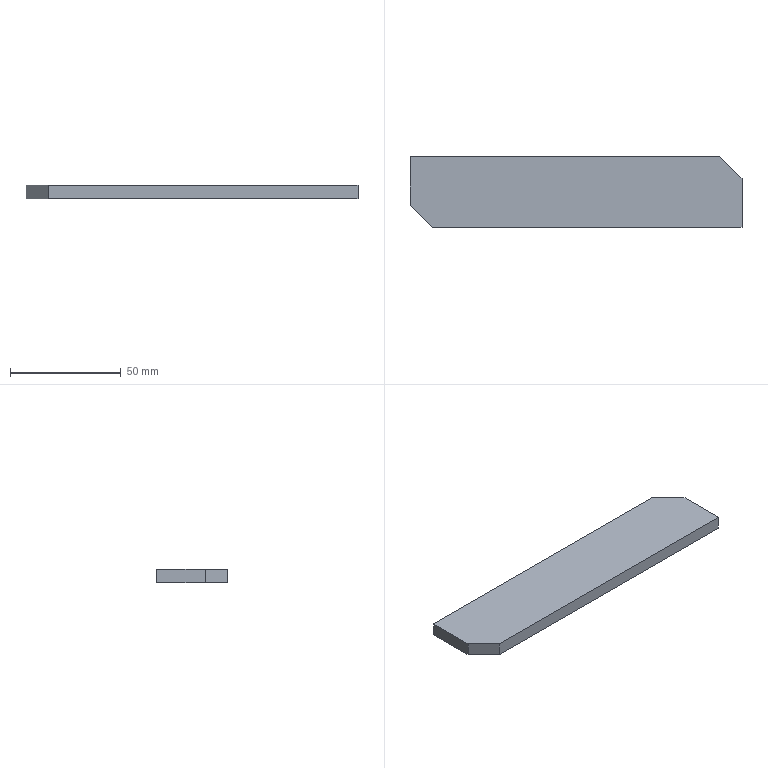Part | STEP file | [02]-7 | 1 solid | 8 faces | box 150 x 32 x 6 mm | volume 28200 mm3 | plane 8
STEP:
#1=CARTESIAN_POINT('',(0.,0.,0.));
#2=DIRECTION('',(0.,0.,1.));
#3=DIRECTION('',(1.,0.,0.));
#4=AXIS2_PLACEMENT_3D('',#1,#2,#3);
#5=CARTESIAN_POINT('',(0.,-22.,0.));
#6=VERTEX_POINT('',#5);
#7=CARTESIAN_POINT('',(0.,0.,0.));
#8=VERTEX_POINT('',#7);
#9=CARTESIAN_POINT('',(0.,-16.,0.));
#10=DIRECTION('',(0.,1.,0.));
#11=VECTOR('',#10,1.);
#12=LINE('',#9,#11);
#13=CARTESIAN_POINT('',(75.,-16.,0.));
#14=DIRECTION('',(0.,0.,-1.));
#15=DIRECTION('',(0.,-1.,0.));
#16=AXIS2_PLACEMENT_3D('',#13,#14,#15);
#17=PLANE('',#16);
#18=CARTESIAN_POINT('',(0.,75.));
#19=DIRECTION('',(-1.,0.));
#20=VECTOR('',#19,1.);
#21=LINE('',#18,#20);
#22=(GEOMETRIC_REPRESENTATION_CONTEXT(2)PARAMETRIC_REPRESENTATION_CONTEXT()REPRESENTATION_CONTEXT('',''));
#23=DEFINITIONAL_REPRESENTATION('',(#21),#22);
#24=PCURVE('',#17,#23);
#25=CARTESIAN_POINT('',(0.,-16.,6.));
#26=DIRECTION('',(-1.,0.,0.));
#27=DIRECTION('',(0.,0.,1.));
#28=AXIS2_PLACEMENT_3D('',#25,#26,#27);
#29=PLANE('',#28);
#30=CARTESIAN_POINT('',(-6.,0.));
#31=DIRECTION('',(0.,1.));
#32=VECTOR('',#31,1.);
#33=LINE('',#30,#32);
#34=(GEOMETRIC_REPRESENTATION_CONTEXT(2)PARAMETRIC_REPRESENTATION_CONTEXT()REPRESENTATION_CONTEXT('',''));
#35=DEFINITIONAL_REPRESENTATION('',(#33),#34);
#36=PCURVE('',#29,#35);
#37=SURFACE_CURVE('',#12,(#24,#36),.PCURVE_S1.);
#38=EDGE_CURVE('',#6,#8,#37,.T.);
#39=ORIENTED_EDGE('',*,*,#38,.T.);
#40=CARTESIAN_POINT('',(140.,0.,0.));
#41=VERTEX_POINT('',#40);
#42=CARTESIAN_POINT('',(75.,0.,0.));
#43=DIRECTION('',(1.,0.,0.));
#44=VECTOR('',#43,1.);
#45=LINE('',#42,#44);
#46=CARTESIAN_POINT('',(-16.,0.));
#47=DIRECTION('',(0.,-1.));
#48=VECTOR('',#47,1.);
#49=LINE('',#46,#48);
#50=(GEOMETRIC_REPRESENTATION_CONTEXT(2)PARAMETRIC_REPRESENTATION_CONTEXT()REPRESENTATION_CONTEXT('',''));
#51=DEFINITIONAL_REPRESENTATION('',(#49),#50);
#52=PCURVE('',#17,#51);
#53=CARTESIAN_POINT('',(75.,0.,6.));
#54=DIRECTION('',(0.,1.,0.));
#55=DIRECTION('',(0.,0.,-1.));
#56=AXIS2_PLACEMENT_3D('',#53,#54,#55);
#57=PLANE('',#56);
#58=CARTESIAN_POINT('',(6.,0.));
#59=DIRECTION('',(0.,-1.));
#60=VECTOR('',#59,1.);
#61=LINE('',#58,#60);
#62=(GEOMETRIC_REPRESENTATION_CONTEXT(2)PARAMETRIC_REPRESENTATION_CONTEXT()REPRESENTATION_CONTEXT('',''));
#63=DEFINITIONAL_REPRESENTATION('',(#61),#62);
#64=PCURVE('',#57,#63);
#65=SURFACE_CURVE('',#45,(#52,#64),.PCURVE_S1.);
#66=EDGE_CURVE('',#8,#41,#65,.T.);
#67=ORIENTED_EDGE('',*,*,#66,.T.);
#68=CARTESIAN_POINT('',(150.,-10.,0.));
#69=VERTEX_POINT('',#68);
#70=CARTESIAN_POINT('',(115.5,24.5,0.));
#71=DIRECTION('',(-0.7071,0.7071,0.));
#72=VECTOR('',#71,1.);
#73=LINE('',#70,#72);
#74=CARTESIAN_POINT('',(-40.5,-40.5));
#75=DIRECTION('',(-0.7071,0.7071));
#76=VECTOR('',#75,1.);
#77=LINE('',#74,#76);
#78=(GEOMETRIC_REPRESENTATION_CONTEXT(2)PARAMETRIC_REPRESENTATION_CONTEXT()REPRESENTATION_CONTEXT('',''));
#79=DEFINITIONAL_REPRESENTATION('',(#77),#78);
#80=PCURVE('',#17,#79);
#81=CARTESIAN_POINT('',(150.,-10.,6.));
#82=DIRECTION('',(-0.7071,-0.7071,0.));
#83=DIRECTION('',(0.,0.,-1.));
#84=AXIS2_PLACEMENT_3D('',#81,#82,#83);
#85=PLANE('',#84);
#86=CARTESIAN_POINT('',(6.,-48.79));
#87=DIRECTION('',(0.,-1.));
#88=VECTOR('',#87,1.);
#89=LINE('',#86,#88);
#90=(GEOMETRIC_REPRESENTATION_CONTEXT(2)PARAMETRIC_REPRESENTATION_CONTEXT()REPRESENTATION_CONTEXT('',''));
#91=DEFINITIONAL_REPRESENTATION('',(#89),#90);
#92=PCURVE('',#85,#91);
#93=SURFACE_CURVE('',#73,(#80,#92),.PCURVE_S1.);
#94=EDGE_CURVE('',#69,#41,#93,.T.);
#95=ORIENTED_EDGE('',*,*,#94,.F.);
#96=CARTESIAN_POINT('',(150.,-32.,0.));
#97=VERTEX_POINT('',#96);
#98=CARTESIAN_POINT('',(150.,-16.,0.));
#99=DIRECTION('',(0.,-1.,0.));
#100=VECTOR('',#99,1.);
#101=LINE('',#98,#100);
#102=CARTESIAN_POINT('',(0.,-75.));
#103=DIRECTION('',(1.,0.));
#104=VECTOR('',#103,1.);
#105=LINE('',#102,#104);
#106=(GEOMETRIC_REPRESENTATION_CONTEXT(2)PARAMETRIC_REPRESENTATION_CONTEXT()REPRESENTATION_CONTEXT('',''));
#107=DEFINITIONAL_REPRESENTATION('',(#105),#106);
#108=PCURVE('',#17,#107);
#109=CARTESIAN_POINT('',(150.,-16.,6.));
#110=DIRECTION('',(1.,0.,0.));
#111=DIRECTION('',(0.,0.,-1.));
#112=AXIS2_PLACEMENT_3D('',#109,#110,#111);
#113=PLANE('',#112);
#114=CARTESIAN_POINT('',(6.,0.));
#115=DIRECTION('',(0.,-1.));
#116=VECTOR('',#115,1.);
#117=LINE('',#114,#116);
#118=(GEOMETRIC_REPRESENTATION_CONTEXT(2)PARAMETRIC_REPRESENTATION_CONTEXT()REPRESENTATION_CONTEXT('',''));
#119=DEFINITIONAL_REPRESENTATION('',(#117),#118);
#120=PCURVE('',#113,#119);
#121=SURFACE_CURVE('',#101,(#108,#120),.PCURVE_S1.);
#122=EDGE_CURVE('',#69,#97,#121,.T.);
#123=ORIENTED_EDGE('',*,*,#122,.T.);
#124=CARTESIAN_POINT('',(10.,-32.,0.));
#125=VERTEX_POINT('',#124);
#126=CARTESIAN_POINT('',(75.,-32.,0.));
#127=DIRECTION('',(-1.,0.,0.));
#128=VECTOR('',#127,1.);
#129=LINE('',#126,#128);
#130=CARTESIAN_POINT('',(16.,0.));
#131=DIRECTION('',(0.,1.));
#132=VECTOR('',#131,1.);
#133=LINE('',#130,#132);
#134=(GEOMETRIC_REPRESENTATION_CONTEXT(2)PARAMETRIC_REPRESENTATION_CONTEXT()REPRESENTATION_CONTEXT('',''));
#135=DEFINITIONAL_REPRESENTATION('',(#133),#134);
#136=PCURVE('',#17,#135);
#137=CARTESIAN_POINT('',(75.,-32.,6.));
#138=DIRECTION('',(0.,-1.,0.));
#139=DIRECTION('',(0.,0.,1.));
#140=AXIS2_PLACEMENT_3D('',#137,#138,#139);
#141=PLANE('',#140);
#142=CARTESIAN_POINT('',(-6.,0.));
#143=DIRECTION('',(0.,1.));
#144=VECTOR('',#143,1.);
#145=LINE('',#142,#144);
#146=(GEOMETRIC_REPRESENTATION_CONTEXT(2)PARAMETRIC_REPRESENTATION_CONTEXT()REPRESENTATION_CONTEXT('',''));
#147=DEFINITIONAL_REPRESENTATION('',(#145),#146);
#148=PCURVE('',#141,#147);
#149=SURFACE_CURVE('',#129,(#136,#148),.PCURVE_S1.);
#150=EDGE_CURVE('',#97,#125,#149,.T.);
#151=ORIENTED_EDGE('',*,*,#150,.T.);
#152=CARTESIAN_POINT('',(34.5,-56.5,0.));
#153=DIRECTION('',(0.7071,-0.7071,0.));
#154=VECTOR('',#153,1.);
#155=LINE('',#152,#154);
#156=CARTESIAN_POINT('',(40.5,40.5));
#157=DIRECTION('',(0.7071,-0.7071));
#158=VECTOR('',#157,1.);
#159=LINE('',#156,#158);
#160=(GEOMETRIC_REPRESENTATION_CONTEXT(2)PARAMETRIC_REPRESENTATION_CONTEXT()REPRESENTATION_CONTEXT('',''));
#161=DEFINITIONAL_REPRESENTATION('',(#159),#160);
#162=PCURVE('',#17,#161);
#163=CARTESIAN_POINT('',(0.,-22.,6.));
#164=DIRECTION('',(0.7071,0.7071,0.));
#165=DIRECTION('',(0.,0.,-1.));
#166=AXIS2_PLACEMENT_3D('',#163,#164,#165);
#167=PLANE('',#166);
#168=CARTESIAN_POINT('',(6.,-48.79));
#169=DIRECTION('',(0.,-1.));
#170=VECTOR('',#169,1.);
#171=LINE('',#168,#170);
#172=(GEOMETRIC_REPRESENTATION_CONTEXT(2)PARAMETRIC_REPRESENTATION_CONTEXT()REPRESENTATION_CONTEXT('',''));
#173=DEFINITIONAL_REPRESENTATION('',(#171),#172);
#174=PCURVE('',#167,#173);
#175=SURFACE_CURVE('',#155,(#162,#174),.PCURVE_S1.);
#176=EDGE_CURVE('',#6,#125,#175,.T.);
#177=ORIENTED_EDGE('',*,*,#176,.F.);
#178=EDGE_LOOP('',(#39,#67,#95,#123,#151,#177));
#179=FACE_BOUND('',#178,.T.);
#180=ADVANCED_FACE('',(#179),#17,.T.);
#181=CARTESIAN_POINT('',(0.,0.,6.));
#182=VERTEX_POINT('',#181);
#183=CARTESIAN_POINT('',(0.,-22.,6.));
#184=VERTEX_POINT('',#183);
#185=CARTESIAN_POINT('',(0.,-16.,6.));
#186=DIRECTION('',(0.,-1.,0.));
#187=VECTOR('',#186,1.);
#188=LINE('',#185,#187);
#189=CARTESIAN_POINT('',(0.,0.));
#190=DIRECTION('',(0.,-1.));
#191=VECTOR('',#190,1.);
#192=LINE('',#189,#191);
#193=(GEOMETRIC_REPRESENTATION_CONTEXT(2)PARAMETRIC_REPRESENTATION_CONTEXT()REPRESENTATION_CONTEXT('',''));
#194=DEFINITIONAL_REPRESENTATION('',(#192),#193);
#195=PCURVE('',#29,#194);
#196=CARTESIAN_POINT('',(75.,-16.,6.));
#197=DIRECTION('',(0.,0.,1.));
#198=DIRECTION('',(0.,1.,0.));
#199=AXIS2_PLACEMENT_3D('',#196,#197,#198);
#200=PLANE('',#199);
#201=CARTESIAN_POINT('',(0.,75.));
#202=DIRECTION('',(-1.,0.));
#203=VECTOR('',#202,1.);
#204=LINE('',#201,#203);
#205=(GEOMETRIC_REPRESENTATION_CONTEXT(2)PARAMETRIC_REPRESENTATION_CONTEXT()REPRESENTATION_CONTEXT('',''));
#206=DEFINITIONAL_REPRESENTATION('',(#204),#205);
#207=PCURVE('',#200,#206);
#208=SURFACE_CURVE('',#188,(#195,#207),.PCURVE_S1.);
#209=EDGE_CURVE('',#182,#184,#208,.T.);
#210=ORIENTED_EDGE('',*,*,#209,.F.);
#211=CARTESIAN_POINT('',(0.,0.,6.));
#212=DIRECTION('',(0.,0.,-1.));
#213=VECTOR('',#212,1.);
#214=LINE('',#211,#213);
#215=CARTESIAN_POINT('',(0.,16.));
#216=DIRECTION('',(-1.,0.));
#217=VECTOR('',#216,1.);
#218=LINE('',#215,#217);
#219=(GEOMETRIC_REPRESENTATION_CONTEXT(2)PARAMETRIC_REPRESENTATION_CONTEXT()REPRESENTATION_CONTEXT('',''));
#220=DEFINITIONAL_REPRESENTATION('',(#218),#219);
#221=PCURVE('',#29,#220);
#222=CARTESIAN_POINT('',(0.,75.));
#223=DIRECTION('',(1.,0.));
#224=VECTOR('',#223,1.);
#225=LINE('',#222,#224);
#226=(GEOMETRIC_REPRESENTATION_CONTEXT(2)PARAMETRIC_REPRESENTATION_CONTEXT()REPRESENTATION_CONTEXT('',''));
#227=DEFINITIONAL_REPRESENTATION('',(#225),#226);
#228=PCURVE('',#57,#227);
#229=SURFACE_CURVE('',#214,(#221,#228),.PCURVE_S1.);
#230=EDGE_CURVE('',#182,#8,#229,.T.);
#231=ORIENTED_EDGE('',*,*,#230,.T.);
#232=ORIENTED_EDGE('',*,*,#38,.F.);
#233=CARTESIAN_POINT('',(0.,-22.,6.));
#234=DIRECTION('',(0.,0.,-1.));
#235=VECTOR('',#234,1.);
#236=LINE('',#233,#235);
#237=CARTESIAN_POINT('',(0.,-6.));
#238=DIRECTION('',(-1.,0.));
#239=VECTOR('',#238,1.);
#240=LINE('',#237,#239);
#241=(GEOMETRIC_REPRESENTATION_CONTEXT(2)PARAMETRIC_REPRESENTATION_CONTEXT()REPRESENTATION_CONTEXT('',''));
#242=DEFINITIONAL_REPRESENTATION('',(#240),#241);
#243=PCURVE('',#29,#242);
#244=CARTESIAN_POINT('',(0.,0.));
#245=DIRECTION('',(1.,0.));
#246=VECTOR('',#245,1.);
#247=LINE('',#244,#246);
#248=(GEOMETRIC_REPRESENTATION_CONTEXT(2)PARAMETRIC_REPRESENTATION_CONTEXT()REPRESENTATION_CONTEXT('',''));
#249=DEFINITIONAL_REPRESENTATION('',(#247),#248);
#250=PCURVE('',#167,#249);
#251=SURFACE_CURVE('',#236,(#243,#250),.PCURVE_S1.);
#252=EDGE_CURVE('',#184,#6,#251,.T.);
#253=ORIENTED_EDGE('',*,*,#252,.F.);
#254=EDGE_LOOP('',(#210,#231,#232,#253));
#255=FACE_BOUND('',#254,.T.);
#256=ADVANCED_FACE('',(#255),#29,.T.);
#257=ORIENTED_EDGE('',*,*,#66,.F.);
#258=ORIENTED_EDGE('',*,*,#230,.F.);
#259=CARTESIAN_POINT('',(140.,0.,6.));
#260=VERTEX_POINT('',#259);
#261=CARTESIAN_POINT('',(75.,0.,6.));
#262=DIRECTION('',(-1.,0.,0.));
#263=VECTOR('',#262,1.);
#264=LINE('',#261,#263);
#265=CARTESIAN_POINT('',(0.,0.));
#266=DIRECTION('',(0.,1.));
#267=VECTOR('',#266,1.);
#268=LINE('',#265,#267);
#269=(GEOMETRIC_REPRESENTATION_CONTEXT(2)PARAMETRIC_REPRESENTATION_CONTEXT()REPRESENTATION_CONTEXT('',''));
#270=DEFINITIONAL_REPRESENTATION('',(#268),#269);
#271=PCURVE('',#57,#270);
#272=CARTESIAN_POINT('',(16.,0.));
#273=DIRECTION('',(0.,1.));
#274=VECTOR('',#273,1.);
#275=LINE('',#272,#274);
#276=(GEOMETRIC_REPRESENTATION_CONTEXT(2)PARAMETRIC_REPRESENTATION_CONTEXT()REPRESENTATION_CONTEXT('',''));
#277=DEFINITIONAL_REPRESENTATION('',(#275),#276);
#278=PCURVE('',#200,#277);
#279=SURFACE_CURVE('',#264,(#271,#278),.PCURVE_S1.);
#280=EDGE_CURVE('',#260,#182,#279,.T.);
#281=ORIENTED_EDGE('',*,*,#280,.F.);
#282=CARTESIAN_POINT('',(140.,0.,6.));
#283=DIRECTION('',(0.,0.,1.));
#284=VECTOR('',#283,1.);
#285=LINE('',#282,#284);
#286=CARTESIAN_POINT('',(0.,-65.));
#287=DIRECTION('',(-1.,0.));
#288=VECTOR('',#287,1.);
#289=LINE('',#286,#288);
#290=(GEOMETRIC_REPRESENTATION_CONTEXT(2)PARAMETRIC_REPRESENTATION_CONTEXT()REPRESENTATION_CONTEXT('',''));
#291=DEFINITIONAL_REPRESENTATION('',(#289),#290);
#292=PCURVE('',#57,#291);
#293=CARTESIAN_POINT('',(0.,-14.142));
#294=DIRECTION('',(-1.,0.));
#295=VECTOR('',#294,1.);
#296=LINE('',#293,#295);
#297=(GEOMETRIC_REPRESENTATION_CONTEXT(2)PARAMETRIC_REPRESENTATION_CONTEXT()REPRESENTATION_CONTEXT('',''));
#298=DEFINITIONAL_REPRESENTATION('',(#296),#297);
#299=PCURVE('',#85,#298);
#300=SURFACE_CURVE('',#285,(#292,#299),.PCURVE_S1.);
#301=EDGE_CURVE('',#41,#260,#300,.T.);
#302=ORIENTED_EDGE('',*,*,#301,.F.);
#303=EDGE_LOOP('',(#257,#258,#281,#302));
#304=FACE_BOUND('',#303,.T.);
#305=ADVANCED_FACE('',(#304),#57,.T.);
#306=CARTESIAN_POINT('',(150.,-32.,6.));
#307=VERTEX_POINT('',#306);
#308=CARTESIAN_POINT('',(150.,-10.,6.));
#309=VERTEX_POINT('',#308);
#310=CARTESIAN_POINT('',(150.,-16.,6.));
#311=DIRECTION('',(0.,1.,0.));
#312=VECTOR('',#311,1.);
#313=LINE('',#310,#312);
#314=CARTESIAN_POINT('',(0.,0.));
#315=DIRECTION('',(0.,1.));
#316=VECTOR('',#315,1.);
#317=LINE('',#314,#316);
#318=(GEOMETRIC_REPRESENTATION_CONTEXT(2)PARAMETRIC_REPRESENTATION_CONTEXT()REPRESENTATION_CONTEXT('',''));
#319=DEFINITIONAL_REPRESENTATION('',(#317),#318);
#320=PCURVE('',#113,#319);
#321=CARTESIAN_POINT('',(0.,-75.));
#322=DIRECTION('',(1.,0.));
#323=VECTOR('',#322,1.);
#324=LINE('',#321,#323);
#325=(GEOMETRIC_REPRESENTATION_CONTEXT(2)PARAMETRIC_REPRESENTATION_CONTEXT()REPRESENTATION_CONTEXT('',''));
#326=DEFINITIONAL_REPRESENTATION('',(#324),#325);
#327=PCURVE('',#200,#326);
#328=SURFACE_CURVE('',#313,(#320,#327),.PCURVE_S1.);
#329=EDGE_CURVE('',#307,#309,#328,.T.);
#330=ORIENTED_EDGE('',*,*,#329,.F.);
#331=CARTESIAN_POINT('',(150.,-32.,6.));
#332=DIRECTION('',(0.,0.,-1.));
#333=VECTOR('',#332,1.);
#334=LINE('',#331,#333);
#335=CARTESIAN_POINT('',(0.,-16.));
#336=DIRECTION('',(1.,0.));
#337=VECTOR('',#336,1.);
#338=LINE('',#335,#337);
#339=(GEOMETRIC_REPRESENTATION_CONTEXT(2)PARAMETRIC_REPRESENTATION_CONTEXT()REPRESENTATION_CONTEXT('',''));
#340=DEFINITIONAL_REPRESENTATION('',(#338),#339);
#341=PCURVE('',#113,#340);
#342=CARTESIAN_POINT('',(0.,-75.));
#343=DIRECTION('',(-1.,0.));
#344=VECTOR('',#343,1.);
#345=LINE('',#342,#344);
#346=(GEOMETRIC_REPRESENTATION_CONTEXT(2)PARAMETRIC_REPRESENTATION_CONTEXT()REPRESENTATION_CONTEXT('',''));
#347=DEFINITIONAL_REPRESENTATION('',(#345),#346);
#348=PCURVE('',#141,#347);
#349=SURFACE_CURVE('',#334,(#341,#348),.PCURVE_S1.);
#350=EDGE_CURVE('',#307,#97,#349,.T.);
#351=ORIENTED_EDGE('',*,*,#350,.T.);
#352=ORIENTED_EDGE('',*,*,#122,.F.);
#353=CARTESIAN_POINT('',(150.,-10.,6.));
#354=DIRECTION('',(0.,0.,-1.));
#355=VECTOR('',#354,1.);
#356=LINE('',#353,#355);
#357=CARTESIAN_POINT('',(0.,6.));
#358=DIRECTION('',(1.,0.));
#359=VECTOR('',#358,1.);
#360=LINE('',#357,#359);
#361=(GEOMETRIC_REPRESENTATION_CONTEXT(2)PARAMETRIC_REPRESENTATION_CONTEXT()REPRESENTATION_CONTEXT('',''));
#362=DEFINITIONAL_REPRESENTATION('',(#360),#361);
#363=PCURVE('',#113,#362);
#364=CARTESIAN_POINT('',(0.,0.));
#365=DIRECTION('',(1.,0.));
#366=VECTOR('',#365,1.);
#367=LINE('',#364,#366);
#368=(GEOMETRIC_REPRESENTATION_CONTEXT(2)PARAMETRIC_REPRESENTATION_CONTEXT()REPRESENTATION_CONTEXT('',''));
#369=DEFINITIONAL_REPRESENTATION('',(#367),#368);
#370=PCURVE('',#85,#369);
#371=SURFACE_CURVE('',#356,(#363,#370),.PCURVE_S1.);
#372=EDGE_CURVE('',#309,#69,#371,.T.);
#373=ORIENTED_EDGE('',*,*,#372,.F.);
#374=EDGE_LOOP('',(#330,#351,#352,#373));
#375=FACE_BOUND('',#374,.T.);
#376=ADVANCED_FACE('',(#375),#113,.T.);
#377=CARTESIAN_POINT('',(10.,-32.,6.));
#378=VERTEX_POINT('',#377);
#379=CARTESIAN_POINT('',(75.,-32.,6.));
#380=DIRECTION('',(1.,0.,0.));
#381=VECTOR('',#380,1.);
#382=LINE('',#379,#381);
#383=CARTESIAN_POINT('',(-16.,0.));
#384=DIRECTION('',(0.,-1.));
#385=VECTOR('',#384,1.);
#386=LINE('',#383,#385);
#387=(GEOMETRIC_REPRESENTATION_CONTEXT(2)PARAMETRIC_REPRESENTATION_CONTEXT()REPRESENTATION_CONTEXT('',''));
#388=DEFINITIONAL_REPRESENTATION('',(#386),#387);
#389=PCURVE('',#200,#388);
#390=CARTESIAN_POINT('',(0.,0.));
#391=DIRECTION('',(0.,-1.));
#392=VECTOR('',#391,1.);
#393=LINE('',#390,#392);
#394=(GEOMETRIC_REPRESENTATION_CONTEXT(2)PARAMETRIC_REPRESENTATION_CONTEXT()REPRESENTATION_CONTEXT('',''));
#395=DEFINITIONAL_REPRESENTATION('',(#393),#394);
#396=PCURVE('',#141,#395);
#397=SURFACE_CURVE('',#382,(#389,#396),.PCURVE_S1.);
#398=EDGE_CURVE('',#378,#307,#397,.T.);
#399=ORIENTED_EDGE('',*,*,#398,.T.);
#400=ORIENTED_EDGE('',*,*,#329,.T.);
#401=CARTESIAN_POINT('',(115.5,24.5,6.));
#402=DIRECTION('',(0.7071,-0.7071,0.));
#403=VECTOR('',#402,1.);
#404=LINE('',#401,#403);
#405=CARTESIAN_POINT('',(40.5,-40.5));
#406=DIRECTION('',(-0.7071,-0.7071));
#407=VECTOR('',#406,1.);
#408=LINE('',#405,#407);
#409=(GEOMETRIC_REPRESENTATION_CONTEXT(2)PARAMETRIC_REPRESENTATION_CONTEXT()REPRESENTATION_CONTEXT('',''));
#410=DEFINITIONAL_REPRESENTATION('',(#408),#409);
#411=PCURVE('',#200,#410);
#412=CARTESIAN_POINT('',(0.,-48.79));
#413=DIRECTION('',(0.,1.));
#414=VECTOR('',#413,1.);
#415=LINE('',#412,#414);
#416=(GEOMETRIC_REPRESENTATION_CONTEXT(2)PARAMETRIC_REPRESENTATION_CONTEXT()REPRESENTATION_CONTEXT('',''));
#417=DEFINITIONAL_REPRESENTATION('',(#415),#416);
#418=PCURVE('',#85,#417);
#419=SURFACE_CURVE('',#404,(#411,#418),.PCURVE_S1.);
#420=EDGE_CURVE('',#260,#309,#419,.T.);
#421=ORIENTED_EDGE('',*,*,#420,.F.);
#422=ORIENTED_EDGE('',*,*,#280,.T.);
#423=ORIENTED_EDGE('',*,*,#209,.T.);
#424=CARTESIAN_POINT('',(34.5,-56.5,6.));
#425=DIRECTION('',(-0.7071,0.7071,0.));
#426=VECTOR('',#425,1.);
#427=LINE('',#424,#426);
#428=CARTESIAN_POINT('',(-40.5,40.5));
#429=DIRECTION('',(0.7071,0.7071));
#430=VECTOR('',#429,1.);
#431=LINE('',#428,#430);
#432=(GEOMETRIC_REPRESENTATION_CONTEXT(2)PARAMETRIC_REPRESENTATION_CONTEXT()REPRESENTATION_CONTEXT('',''));
#433=DEFINITIONAL_REPRESENTATION('',(#431),#432);
#434=PCURVE('',#200,#433);
#435=CARTESIAN_POINT('',(0.,-48.79));
#436=DIRECTION('',(0.,1.));
#437=VECTOR('',#436,1.);
#438=LINE('',#435,#437);
#439=(GEOMETRIC_REPRESENTATION_CONTEXT(2)PARAMETRIC_REPRESENTATION_CONTEXT()REPRESENTATION_CONTEXT('',''));
#440=DEFINITIONAL_REPRESENTATION('',(#438),#439);
#441=PCURVE('',#167,#440);
#442=SURFACE_CURVE('',#427,(#434,#441),.PCURVE_S1.);
#443=EDGE_CURVE('',#378,#184,#442,.T.);
#444=ORIENTED_EDGE('',*,*,#443,.F.);
#445=EDGE_LOOP('',(#399,#400,#421,#422,#423,#444));
#446=FACE_BOUND('',#445,.T.);
#447=ADVANCED_FACE('',(#446),#200,.T.);
#448=ORIENTED_EDGE('',*,*,#150,.F.);
#449=ORIENTED_EDGE('',*,*,#350,.F.);
#450=ORIENTED_EDGE('',*,*,#398,.F.);
#451=CARTESIAN_POINT('',(10.,-32.,6.));
#452=DIRECTION('',(0.,0.,1.));
#453=VECTOR('',#452,1.);
#454=LINE('',#451,#453);
#455=CARTESIAN_POINT('',(0.,65.));
#456=DIRECTION('',(1.,0.));
#457=VECTOR('',#456,1.);
#458=LINE('',#455,#457);
#459=(GEOMETRIC_REPRESENTATION_CONTEXT(2)PARAMETRIC_REPRESENTATION_CONTEXT()REPRESENTATION_CONTEXT('',''));
#460=DEFINITIONAL_REPRESENTATION('',(#458),#459);
#461=PCURVE('',#141,#460);
#462=CARTESIAN_POINT('',(0.,-14.142));
#463=DIRECTION('',(-1.,0.));
#464=VECTOR('',#463,1.);
#465=LINE('',#462,#464);
#466=(GEOMETRIC_REPRESENTATION_CONTEXT(2)PARAMETRIC_REPRESENTATION_CONTEXT()REPRESENTATION_CONTEXT('',''));
#467=DEFINITIONAL_REPRESENTATION('',(#465),#466);
#468=PCURVE('',#167,#467);
#469=SURFACE_CURVE('',#454,(#461,#468),.PCURVE_S1.);
#470=EDGE_CURVE('',#125,#378,#469,.T.);
#471=ORIENTED_EDGE('',*,*,#470,.F.);
#472=EDGE_LOOP('',(#448,#449,#450,#471));
#473=FACE_BOUND('',#472,.T.);
#474=ADVANCED_FACE('',(#473),#141,.T.);
#475=ORIENTED_EDGE('',*,*,#420,.T.);
#476=ORIENTED_EDGE('',*,*,#372,.T.);
#477=ORIENTED_EDGE('',*,*,#94,.T.);
#478=ORIENTED_EDGE('',*,*,#301,.T.);
#479=EDGE_LOOP('',(#475,#476,#477,#478));
#480=FACE_BOUND('',#479,.T.);
#481=ADVANCED_FACE('',(#480),#85,.F.);
#482=ORIENTED_EDGE('',*,*,#443,.T.);
#483=ORIENTED_EDGE('',*,*,#252,.T.);
#484=ORIENTED_EDGE('',*,*,#176,.T.);
#485=ORIENTED_EDGE('',*,*,#470,.T.);
#486=EDGE_LOOP('',(#482,#483,#484,#485));
#487=FACE_BOUND('',#486,.T.);
#488=ADVANCED_FACE('',(#487),#167,.F.);
#489=CLOSED_SHELL('',(#180,#256,#305,#376,#447,#474,#481,#488));
#490=MANIFOLD_SOLID_BREP('',#489);
#491=(LENGTH_UNIT()NAMED_UNIT(*)SI_UNIT(.MILLI.,.METRE.));
#492=UNCERTAINTY_MEASURE_WITH_UNIT(LENGTH_MEASURE(0.0000001),#491,'','');
#493=(NAMED_UNIT(*)PLANE_ANGLE_UNIT()SI_UNIT($,.RADIAN.));
#494=(NAMED_UNIT(*)SI_UNIT($,.STERADIAN.)SOLID_ANGLE_UNIT());
#495=(GEOMETRIC_REPRESENTATION_CONTEXT(3)GLOBAL_UNCERTAINTY_ASSIGNED_CONTEXT((#492))GLOBAL_UNIT_ASSIGNED_CONTEXT((#491,#493,#494))REPRESENTATION_CONTEXT('',''));
#496=ADVANCED_BREP_SHAPE_REPRESENTATION('',(#4,#490),#495);